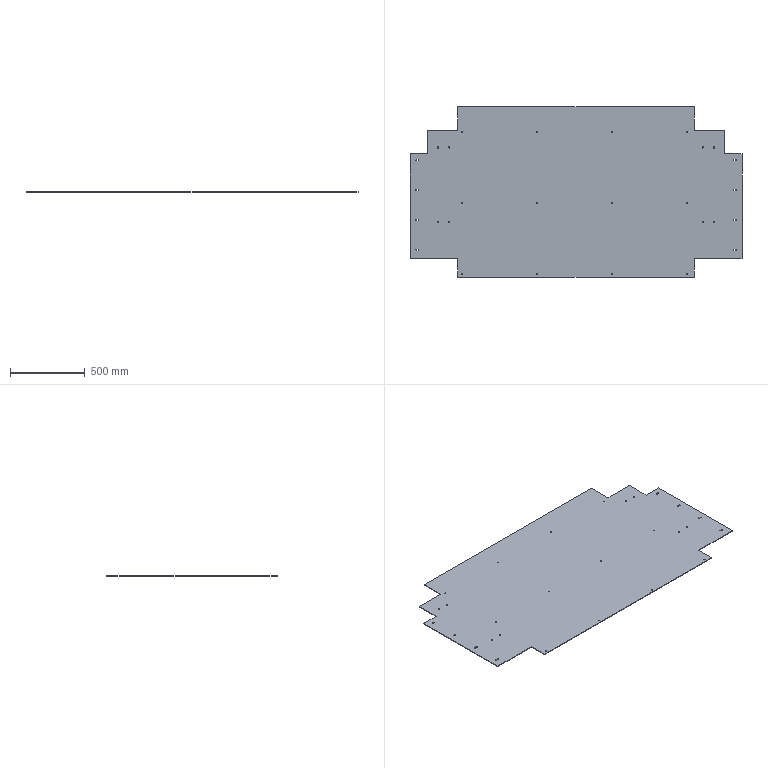Part | SolidWorks | features Extrusion 1, ICE 1 | 1 solid | 98 faces | box 2220 x 1140 x 4 mm | volume 9243673 mm3 | cylinder 64 | plane 34 | commonest cylinder face diameters 9 x40 7 x24